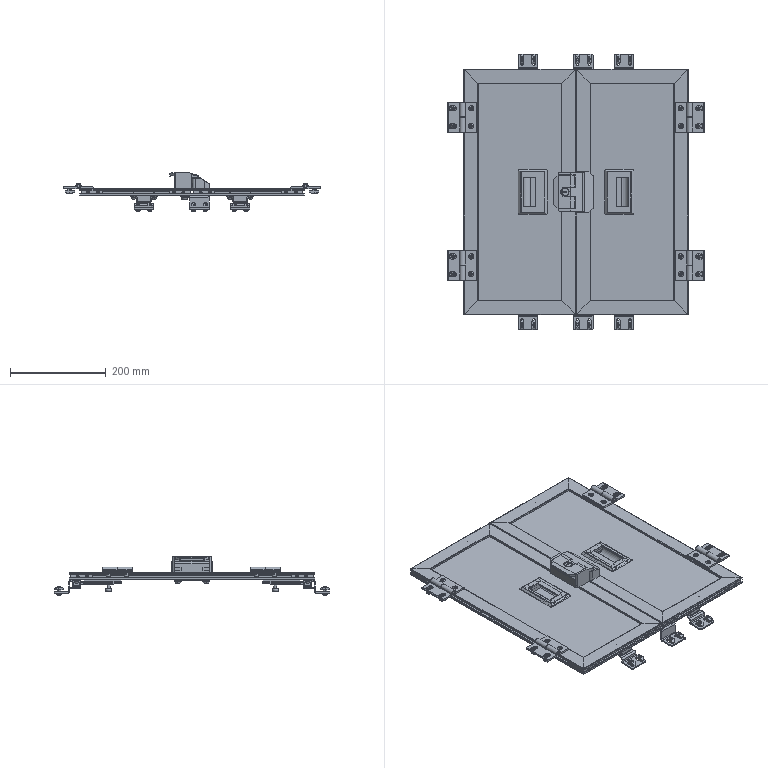Part | NX | features BREP 38 | 204 solids | 4844 faces | volume 1932834 mm3 | plane 2683 | cylinder 1465 | cone 560 | torus 102 | sphere 34 | commonest cylinder face diameters 5 x396 6 x114 8 x108 4 x101 1 x87 2 x73